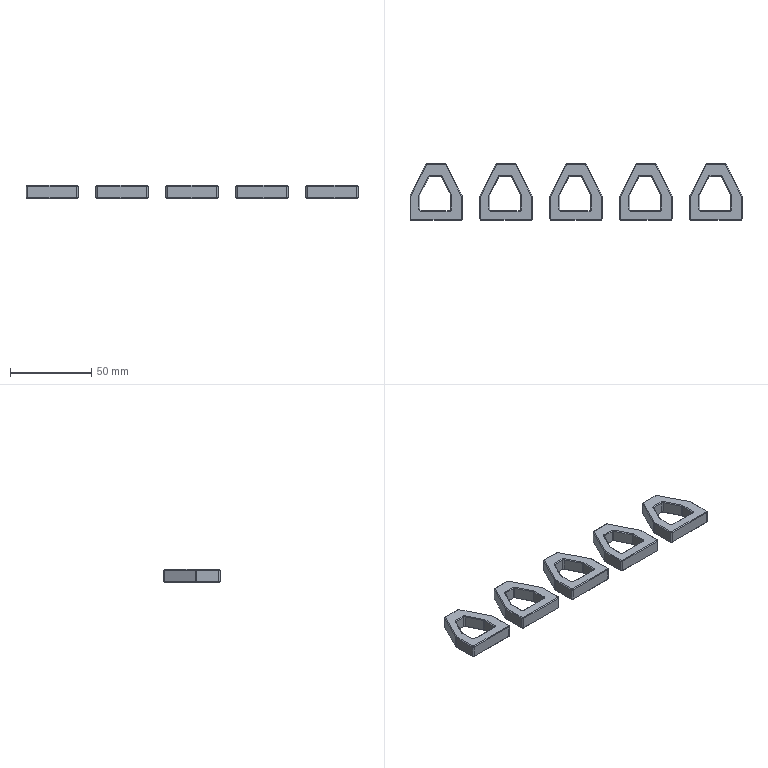NC program | NX | posted with a generic post | part box 204 x 35 x 8 mm
Lines 1 to 18 of 15564:
N10 G17 G21 G94 G90
(FLOOR_WALL , TOOL : D80)
N12 T19 M6
N14 G54
N16 G17 G0 G90 X-147. Y0. S6500 M3
N18 G43 Z30. H19
N20 Z3.
N22 G94 G1 Z0. F1500.
N24 X-144.
N26 X144.
N28 X147.
N30 Z3.
N32 G0 Z30.
N34 M5